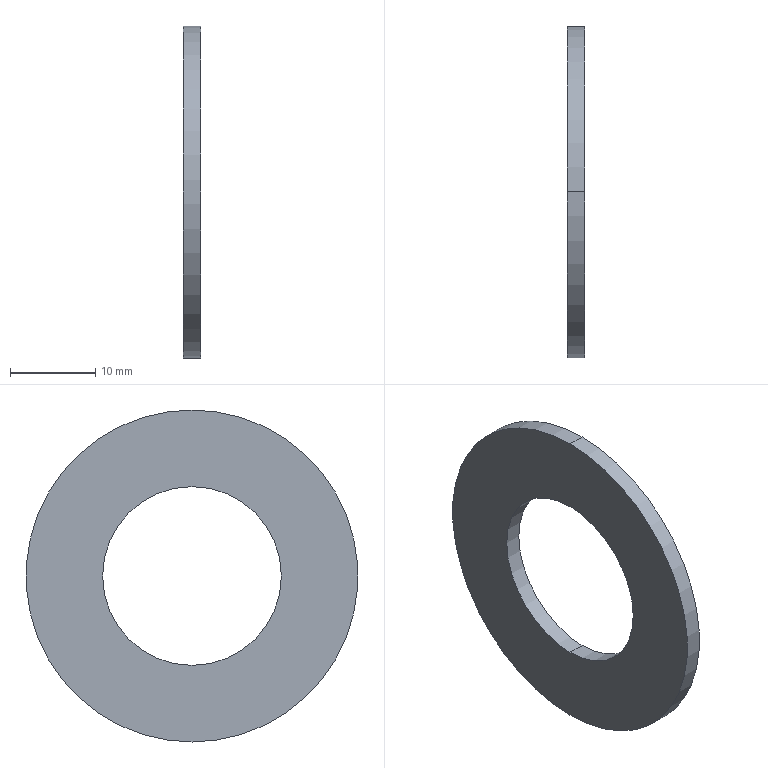Part | NX | features BREP 1 | 1 solid | 6 faces | box 2 x 39 x 39 mm | volume 1696 mm3 | cylinder 4 | plane 2 | commonest cylinder face diameters 21 x2 39 x2
STEP:
#1=CARTESIAN_POINT('',(683.955,24.898,70.542));
#2=VERTEX_POINT('',#1);
#3=CARTESIAN_POINT('',(683.955,24.898,49.542));
#4=VERTEX_POINT('',#3);
#5=CARTESIAN_POINT('',(683.955,24.898,60.042));
#6=DIRECTION('',(1.,0.,0.));
#7=DIRECTION('',(0.,0.,-1.));
#8=AXIS2_PLACEMENT_3D('',#5,#6,#7);
#9=CIRCLE('',#8,10.5);
#10=EDGE_CURVE('',#2,#4,#9,.T.);
#11=ORIENTED_EDGE('',*,*,#10,.F.);
#12=CARTESIAN_POINT('',(683.955,24.898,60.042));
#13=DIRECTION('',(1.,0.,0.));
#14=DIRECTION('',(0.,0.,-1.));
#15=AXIS2_PLACEMENT_3D('',#12,#13,#14);
#16=CIRCLE('',#15,10.5);
#17=EDGE_CURVE('',#4,#2,#16,.T.);
#18=ORIENTED_EDGE('',*,*,#17,.F.);
#19=EDGE_LOOP('',(#11,#18));
#20=FACE_BOUND('',#19,.T.);
#21=CARTESIAN_POINT('',(683.955,24.898,79.542));
#22=VERTEX_POINT('',#21);
#23=CARTESIAN_POINT('',(683.955,24.898,40.542));
#24=VERTEX_POINT('',#23);
#25=CARTESIAN_POINT('',(683.955,24.898,60.042));
#26=DIRECTION('',(1.,0.,0.));
#27=DIRECTION('',(0.,0.,-1.));
#28=AXIS2_PLACEMENT_3D('',#25,#26,#27);
#29=CIRCLE('',#28,19.5);
#30=EDGE_CURVE('',#22,#24,#29,.T.);
#31=ORIENTED_EDGE('',*,*,#30,.T.);
#32=CARTESIAN_POINT('',(683.955,24.898,60.042));
#33=DIRECTION('',(1.,0.,0.));
#34=DIRECTION('',(0.,0.,-1.));
#35=AXIS2_PLACEMENT_3D('',#32,#33,#34);
#36=CIRCLE('',#35,19.5);
#37=EDGE_CURVE('',#24,#22,#36,.T.);
#38=ORIENTED_EDGE('',*,*,#37,.T.);
#39=EDGE_LOOP('',(#31,#38));
#40=FACE_BOUND('',#39,.T.);
#41=CARTESIAN_POINT('',(683.955,24.898,60.042));
#42=DIRECTION('',(1.,0.,0.));
#43=DIRECTION('',(0.,0.,1.));
#44=AXIS2_PLACEMENT_3D('',#41,#42,#43);
#45=PLANE('',#44);
#46=ADVANCED_FACE('',(#20,#40),#45,.T.);
#47=CARTESIAN_POINT('',(681.955,24.898,70.542));
#48=VERTEX_POINT('',#47);
#49=CARTESIAN_POINT('',(681.955,24.898,49.542));
#50=VERTEX_POINT('',#49);
#51=CARTESIAN_POINT('',(681.955,24.898,60.042));
#52=DIRECTION('',(1.,0.,0.));
#53=DIRECTION('',(0.,0.,-1.));
#54=AXIS2_PLACEMENT_3D('',#51,#52,#53);
#55=CIRCLE('',#54,10.5);
#56=EDGE_CURVE('',#48,#50,#55,.T.);
#57=ORIENTED_EDGE('',*,*,#56,.T.);
#58=CARTESIAN_POINT('',(681.955,24.898,60.042));
#59=DIRECTION('',(1.,0.,0.));
#60=DIRECTION('',(0.,0.,-1.));
#61=AXIS2_PLACEMENT_3D('',#58,#59,#60);
#62=CIRCLE('',#61,10.5);
#63=EDGE_CURVE('',#50,#48,#62,.T.);
#64=ORIENTED_EDGE('',*,*,#63,.T.);
#65=EDGE_LOOP('',(#57,#64));
#66=FACE_BOUND('',#65,.T.);
#67=CARTESIAN_POINT('',(681.955,24.898,79.542));
#68=VERTEX_POINT('',#67);
#69=CARTESIAN_POINT('',(681.955,24.898,40.542));
#70=VERTEX_POINT('',#69);
#71=CARTESIAN_POINT('',(681.955,24.898,60.042));
#72=DIRECTION('',(1.,0.,0.));
#73=DIRECTION('',(0.,0.,-1.));
#74=AXIS2_PLACEMENT_3D('',#71,#72,#73);
#75=CIRCLE('',#74,19.5);
#76=EDGE_CURVE('',#68,#70,#75,.T.);
#77=ORIENTED_EDGE('',*,*,#76,.F.);
#78=CARTESIAN_POINT('',(681.955,24.898,60.042));
#79=DIRECTION('',(1.,0.,0.));
#80=DIRECTION('',(0.,0.,-1.));
#81=AXIS2_PLACEMENT_3D('',#78,#79,#80);
#82=CIRCLE('',#81,19.5);
#83=EDGE_CURVE('',#70,#68,#82,.T.);
#84=ORIENTED_EDGE('',*,*,#83,.F.);
#85=EDGE_LOOP('',(#77,#84));
#86=FACE_BOUND('',#85,.T.);
#87=CARTESIAN_POINT('',(681.955,24.898,60.042));
#88=DIRECTION('',(1.,0.,0.));
#89=DIRECTION('',(0.,0.,1.));
#90=AXIS2_PLACEMENT_3D('',#87,#88,#89);
#91=PLANE('',#90);
#92=ADVANCED_FACE('',(#66,#86),#91,.F.);
#93=CARTESIAN_POINT('',(683.955,24.898,40.542));
#94=DIRECTION('',(-1.,0.,0.));
#95=VECTOR('',#94,1000.);
#96=LINE('',#93,#95);
#97=EDGE_CURVE('',#24,#70,#96,.T.);
#98=ORIENTED_EDGE('',*,*,#97,.T.);
#99=ORIENTED_EDGE('',*,*,#83,.T.);
#100=CARTESIAN_POINT('',(683.955,24.898,79.542));
#101=DIRECTION('',(-1.,0.,0.));
#102=VECTOR('',#101,1000.);
#103=LINE('',#100,#102);
#104=EDGE_CURVE('',#22,#68,#103,.T.);
#105=ORIENTED_EDGE('',*,*,#104,.F.);
#106=ORIENTED_EDGE('',*,*,#37,.F.);
#107=EDGE_LOOP('',(#98,#99,#105,#106));
#108=FACE_BOUND('',#107,.T.);
#109=CARTESIAN_POINT('',(683.955,24.898,60.042));
#110=DIRECTION('',(1.,0.,0.));
#111=DIRECTION('',(0.,0.,-1.));
#112=AXIS2_PLACEMENT_3D('',#109,#110,#111);
#113=CYLINDRICAL_SURFACE('',#112,19.5);
#114=ADVANCED_FACE('',(#108),#113,.T.);
#115=CARTESIAN_POINT('',(683.955,24.898,49.542));
#116=DIRECTION('',(-1.,0.,0.));
#117=VECTOR('',#116,1000.);
#118=LINE('',#115,#117);
#119=EDGE_CURVE('',#4,#50,#118,.T.);
#120=ORIENTED_EDGE('',*,*,#119,.T.);
#121=ORIENTED_EDGE('',*,*,#56,.F.);
#122=CARTESIAN_POINT('',(683.955,24.898,70.542));
#123=DIRECTION('',(-1.,0.,0.));
#124=VECTOR('',#123,1000.);
#125=LINE('',#122,#124);
#126=EDGE_CURVE('',#2,#48,#125,.T.);
#127=ORIENTED_EDGE('',*,*,#126,.F.);
#128=ORIENTED_EDGE('',*,*,#10,.T.);
#129=EDGE_LOOP('',(#120,#121,#127,#128));
#130=FACE_BOUND('',#129,.T.);
#131=CARTESIAN_POINT('',(683.955,24.898,60.042));
#132=DIRECTION('',(1.,0.,0.));
#133=DIRECTION('',(0.,0.,-1.));
#134=AXIS2_PLACEMENT_3D('',#131,#132,#133);
#135=CYLINDRICAL_SURFACE('',#134,10.5);
#136=ADVANCED_FACE('',(#130),#135,.F.);
#137=ORIENTED_EDGE('',*,*,#63,.F.);
#138=ORIENTED_EDGE('',*,*,#119,.F.);
#139=ORIENTED_EDGE('',*,*,#17,.T.);
#140=ORIENTED_EDGE('',*,*,#126,.T.);
#141=EDGE_LOOP('',(#137,#138,#139,#140));
#142=FACE_BOUND('',#141,.T.);
#143=CARTESIAN_POINT('',(683.955,24.898,60.042));
#144=DIRECTION('',(1.,0.,0.));
#145=DIRECTION('',(0.,0.,-1.));
#146=AXIS2_PLACEMENT_3D('',#143,#144,#145);
#147=CYLINDRICAL_SURFACE('',#146,10.5);
#148=ADVANCED_FACE('',(#142),#147,.F.);
#149=ORIENTED_EDGE('',*,*,#76,.T.);
#150=ORIENTED_EDGE('',*,*,#97,.F.);
#151=ORIENTED_EDGE('',*,*,#30,.F.);
#152=ORIENTED_EDGE('',*,*,#104,.T.);
#153=EDGE_LOOP('',(#149,#150,#151,#152));
#154=FACE_BOUND('',#153,.T.);
#155=CARTESIAN_POINT('',(683.955,24.898,60.042));
#156=DIRECTION('',(1.,0.,0.));
#157=DIRECTION('',(0.,0.,-1.));
#158=AXIS2_PLACEMENT_3D('',#155,#156,#157);
#159=CYLINDRICAL_SURFACE('',#158,19.5);
#160=ADVANCED_FACE('',(#154),#159,.T.);
#161=CLOSED_SHELL('',(#46,#92,#114,#136,#148,#160));
#162=MANIFOLD_SOLID_BREP('',#161);
#163=(LENGTH_UNIT()NAMED_UNIT(*)SI_UNIT(.MILLI.,.METRE.));
#164=UNCERTAINTY_MEASURE_WITH_UNIT(LENGTH_MEASURE(0.00001),#163,'','');
#165=(NAMED_UNIT(*)PLANE_ANGLE_UNIT()SI_UNIT($,.RADIAN.));
#166=(NAMED_UNIT(*)SI_UNIT($,.STERADIAN.)SOLID_ANGLE_UNIT());
#167=(GEOMETRIC_REPRESENTATION_CONTEXT(3)GLOBAL_UNCERTAINTY_ASSIGNED_CONTEXT((#164))GLOBAL_UNIT_ASSIGNED_CONTEXT((#163,#165,#166))REPRESENTATION_CONTEXT('',''));
#168=ADVANCED_BREP_SHAPE_REPRESENTATION('',(#162),#167);